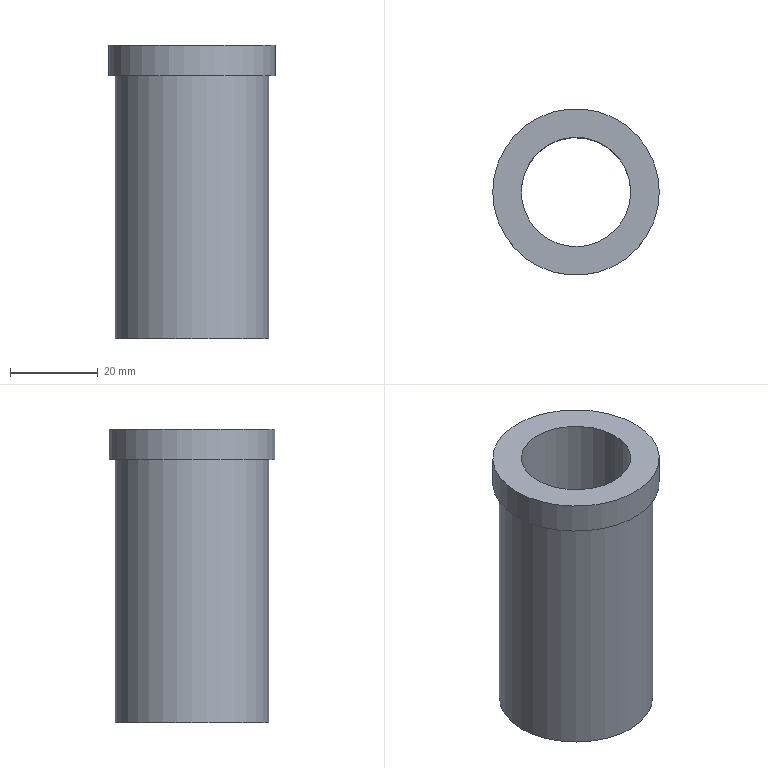Part | STEP file | lll_id578_x_t | 1 solid | 6 faces | box 38 x 38 x 67 mm | volume 32777 mm3 | plane 3 | cylinder 3 | commonest cylinder face diameters 25 x1 35 x1 38 x1
STEP:
#1=CARTESIAN_POINT('',(-84.5,-117.,99.5));
#2=VERTEX_POINT('',#1);
#3=CARTESIAN_POINT('',(-97.,-117.,99.5));
#4=DIRECTION('',(0.,0.,1.));
#5=DIRECTION('',(1.,0.,0.));
#6=AXIS2_PLACEMENT_3D('',#3,#4,#5);
#7=CIRCLE('',#6,12.5);
#8=EDGE_CURVE('',#2,#2,#7,.T.);
#9=ORIENTED_EDGE('',*,*,#8,.F.);
#10=EDGE_LOOP('',(#9));
#11=FACE_BOUND('',#10,.T.);
#12=CARTESIAN_POINT('',(-78.,-117.,99.5));
#13=VERTEX_POINT('',#12);
#14=CARTESIAN_POINT('',(-97.,-117.,99.5));
#15=DIRECTION('',(0.,0.,1.));
#16=DIRECTION('',(1.,0.,0.));
#17=AXIS2_PLACEMENT_3D('',#14,#15,#16);
#18=CIRCLE('',#17,19.);
#19=EDGE_CURVE('',#13,#13,#18,.T.);
#20=ORIENTED_EDGE('',*,*,#19,.T.);
#21=EDGE_LOOP('',(#20));
#22=FACE_BOUND('',#21,.T.);
#23=CARTESIAN_POINT('',(0.,0.,99.5));
#24=DIRECTION('',(0.,0.,1.));
#25=DIRECTION('',(1.,0.,0.));
#26=AXIS2_PLACEMENT_3D('',#23,#24,#25);
#27=PLANE('',#26);
#28=ADVANCED_FACE('',(#11,#22),#27,.T.);
#29=CARTESIAN_POINT('',(-78.,-117.,92.5));
#30=VERTEX_POINT('',#29);
#31=CARTESIAN_POINT('',(-97.,-117.,92.5));
#32=DIRECTION('',(0.,0.,1.));
#33=DIRECTION('',(1.,0.,0.));
#34=AXIS2_PLACEMENT_3D('',#31,#32,#33);
#35=CIRCLE('',#34,19.);
#36=EDGE_CURVE('',#30,#30,#35,.T.);
#37=ORIENTED_EDGE('',*,*,#36,.T.);
#38=EDGE_LOOP('',(#37));
#39=FACE_BOUND('',#38,.T.);
#40=ORIENTED_EDGE('',*,*,#19,.F.);
#41=EDGE_LOOP('',(#40));
#42=FACE_BOUND('',#41,.T.);
#43=CARTESIAN_POINT('',(-97.,-117.,100.5));
#44=DIRECTION('',(0.,0.,-1.));
#45=DIRECTION('',(1.,0.,0.));
#46=AXIS2_PLACEMENT_3D('',#43,#44,#45);
#47=CYLINDRICAL_SURFACE('',#46,19.);
#48=ADVANCED_FACE('',(#39,#42),#47,.T.);
#49=CARTESIAN_POINT('',(-79.5,-117.,92.5));
#50=VERTEX_POINT('',#49);
#51=CARTESIAN_POINT('',(-97.,-117.,92.5));
#52=DIRECTION('',(0.,0.,1.));
#53=DIRECTION('',(1.,0.,0.));
#54=AXIS2_PLACEMENT_3D('',#51,#52,#53);
#55=CIRCLE('',#54,17.5);
#56=EDGE_CURVE('',#50,#50,#55,.T.);
#57=ORIENTED_EDGE('',*,*,#56,.T.);
#58=EDGE_LOOP('',(#57));
#59=FACE_BOUND('',#58,.T.);
#60=ORIENTED_EDGE('',*,*,#36,.F.);
#61=EDGE_LOOP('',(#60));
#62=FACE_BOUND('',#61,.T.);
#63=CARTESIAN_POINT('',(-97.,-117.,92.5));
#64=DIRECTION('',(0.,0.,1.));
#65=DIRECTION('',(1.,0.,0.));
#66=AXIS2_PLACEMENT_3D('',#63,#64,#65);
#67=PLANE('',#66);
#68=ADVANCED_FACE('',(#59,#62),#67,.F.);
#69=CARTESIAN_POINT('',(-79.5,-117.,32.5));
#70=VERTEX_POINT('',#69);
#71=CARTESIAN_POINT('',(-97.,-117.,32.5));
#72=DIRECTION('',(0.,0.,1.));
#73=DIRECTION('',(1.,0.,0.));
#74=AXIS2_PLACEMENT_3D('',#71,#72,#73);
#75=CIRCLE('',#74,17.5);
#76=EDGE_CURVE('',#70,#70,#75,.T.);
#77=ORIENTED_EDGE('',*,*,#76,.T.);
#78=EDGE_LOOP('',(#77));
#79=FACE_BOUND('',#78,.T.);
#80=ORIENTED_EDGE('',*,*,#56,.F.);
#81=EDGE_LOOP('',(#80));
#82=FACE_BOUND('',#81,.T.);
#83=CARTESIAN_POINT('',(-97.,-117.,32.5));
#84=DIRECTION('',(0.,0.,1.));
#85=DIRECTION('',(1.,0.,0.));
#86=AXIS2_PLACEMENT_3D('',#83,#84,#85);
#87=CYLINDRICAL_SURFACE('',#86,17.5);
#88=ADVANCED_FACE('',(#79,#82),#87,.T.);
#89=CARTESIAN_POINT('',(-84.5,-117.,32.5));
#90=VERTEX_POINT('',#89);
#91=CARTESIAN_POINT('',(-97.,-117.,32.5));
#92=DIRECTION('',(0.,0.,1.));
#93=DIRECTION('',(1.,0.,0.));
#94=AXIS2_PLACEMENT_3D('',#91,#92,#93);
#95=CIRCLE('',#94,12.5);
#96=EDGE_CURVE('',#90,#90,#95,.T.);
#97=ORIENTED_EDGE('',*,*,#96,.T.);
#98=EDGE_LOOP('',(#97));
#99=FACE_BOUND('',#98,.T.);
#100=ORIENTED_EDGE('',*,*,#76,.F.);
#101=EDGE_LOOP('',(#100));
#102=FACE_BOUND('',#101,.T.);
#103=CARTESIAN_POINT('',(-97.,-117.,32.5));
#104=DIRECTION('',(0.,0.,1.));
#105=DIRECTION('',(1.,0.,0.));
#106=AXIS2_PLACEMENT_3D('',#103,#104,#105);
#107=PLANE('',#106);
#108=ADVANCED_FACE('',(#99,#102),#107,.F.);
#109=ORIENTED_EDGE('',*,*,#8,.T.);
#110=EDGE_LOOP('',(#109));
#111=FACE_BOUND('',#110,.T.);
#112=ORIENTED_EDGE('',*,*,#96,.F.);
#113=EDGE_LOOP('',(#112));
#114=FACE_BOUND('',#113,.T.);
#115=CARTESIAN_POINT('',(-97.,-117.,-2420.589));
#116=DIRECTION('',(0.,0.,1.));
#117=DIRECTION('',(1.,0.,0.));
#118=AXIS2_PLACEMENT_3D('',#115,#116,#117);
#119=CYLINDRICAL_SURFACE('',#118,12.5);
#120=ADVANCED_FACE('',(#111,#114),#119,.F.);
#121=CLOSED_SHELL('',(#28,#48,#68,#88,#108,#120));
#122=MANIFOLD_SOLID_BREP('',#121);
#123=(LENGTH_UNIT()NAMED_UNIT(*)SI_UNIT(.MILLI.,.METRE.));
#124=UNCERTAINTY_MEASURE_WITH_UNIT(LENGTH_MEASURE(0.00002),#123,'','');
#125=(NAMED_UNIT(*)PLANE_ANGLE_UNIT()SI_UNIT($,.RADIAN.));
#126=PLANE_ANGLE_MEASURE_WITH_UNIT(PLANE_ANGLE_MEASURE(0.01745),#125);
#127=DIMENSIONAL_EXPONENTS(0.,0.,0.,0.,0.,0.,0.);
#128=(CONVERSION_BASED_UNIT('DEGREE',#126)NAMED_UNIT(#127)PLANE_ANGLE_UNIT());
#129=(NAMED_UNIT(*)SI_UNIT($,.STERADIAN.)SOLID_ANGLE_UNIT());
#130=(GEOMETRIC_REPRESENTATION_CONTEXT(3)GLOBAL_UNCERTAINTY_ASSIGNED_CONTEXT((#124))GLOBAL_UNIT_ASSIGNED_CONTEXT((#123,#128,#129))REPRESENTATION_CONTEXT('',''));
#131=ADVANCED_BREP_SHAPE_REPRESENTATION('',(#122),#130);